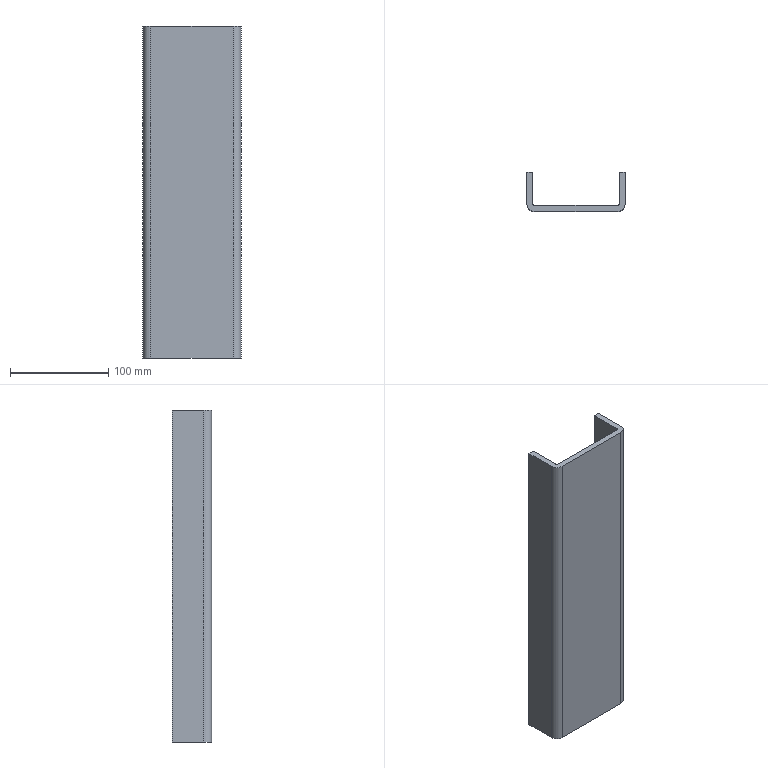Part | SolidWorks | features Extrusion 1 | 1 solid | 14 faces | box 100 x 40 x 337.5 mm | volume 331509 mm3 | plane 10 | cylinder 4 | commonest cylinder face diameters 4 x2 16 x2
STEP:
#1=CARTESIAN_POINT('',(100.,-32.,0.));
#2=VERTEX_POINT('',#1);
#3=CARTESIAN_POINT('',(100.,0.,0.));
#4=VERTEX_POINT('',#3);
#5=CARTESIAN_POINT('',(100.,-32.,0.));
#6=DIRECTION('',(0.,1.,0.));
#7=VECTOR('',#6,1000.);
#8=LINE('',#5,#7);
#9=EDGE_CURVE('',#2,#4,#8,.T.);
#10=ORIENTED_EDGE('',*,*,#9,.T.);
#11=CARTESIAN_POINT('',(100.,0.,337.5));
#12=VERTEX_POINT('',#11);
#13=CARTESIAN_POINT('',(100.,0.,337.5));
#14=DIRECTION('',(0.,0.,-1.));
#15=VECTOR('',#14,1000.);
#16=LINE('',#13,#15);
#17=EDGE_CURVE('',#12,#4,#16,.T.);
#18=ORIENTED_EDGE('',*,*,#17,.F.);
#19=CARTESIAN_POINT('',(100.,-32.,337.5));
#20=VERTEX_POINT('',#19);
#21=CARTESIAN_POINT('',(100.,-32.,337.5));
#22=DIRECTION('',(0.,1.,0.));
#23=VECTOR('',#22,1000.);
#24=LINE('',#21,#23);
#25=EDGE_CURVE('',#20,#12,#24,.T.);
#26=ORIENTED_EDGE('',*,*,#25,.F.);
#27=CARTESIAN_POINT('',(100.,-32.,337.5));
#28=DIRECTION('',(0.,0.,-1.));
#29=VECTOR('',#28,1000.);
#30=LINE('',#27,#29);
#31=EDGE_CURVE('',#20,#2,#30,.T.);
#32=ORIENTED_EDGE('',*,*,#31,.T.);
#33=EDGE_LOOP('',(#10,#18,#26,#32));
#34=FACE_OUTER_BOUND('',#33,.T.);
#35=CARTESIAN_POINT('',(100.,-32.,337.5));
#36=DIRECTION('',(-1.,0.,0.));
#37=DIRECTION('',(0.,0.,1.));
#38=AXIS2_PLACEMENT_3D('',#35,#36,#37);
#39=PLANE('',#38);
#40=ADVANCED_FACE('',(#34),#39,.F.);
#41=CARTESIAN_POINT('',(94.,0.,0.));
#42=VERTEX_POINT('',#41);
#43=CARTESIAN_POINT('',(100.,0.,0.));
#44=DIRECTION('',(-1.,0.,0.));
#45=VECTOR('',#44,1000.);
#46=LINE('',#43,#45);
#47=EDGE_CURVE('',#4,#42,#46,.T.);
#48=ORIENTED_EDGE('',*,*,#47,.T.);
#49=CARTESIAN_POINT('',(94.,0.,337.5));
#50=VERTEX_POINT('',#49);
#51=CARTESIAN_POINT('',(94.,0.,337.5));
#52=DIRECTION('',(0.,0.,-1.));
#53=VECTOR('',#52,1000.);
#54=LINE('',#51,#53);
#55=EDGE_CURVE('',#50,#42,#54,.T.);
#56=ORIENTED_EDGE('',*,*,#55,.F.);
#57=CARTESIAN_POINT('',(100.,0.,337.5));
#58=DIRECTION('',(-1.,0.,0.));
#59=VECTOR('',#58,1000.);
#60=LINE('',#57,#59);
#61=EDGE_CURVE('',#12,#50,#60,.T.);
#62=ORIENTED_EDGE('',*,*,#61,.F.);
#63=ORIENTED_EDGE('',*,*,#17,.T.);
#64=EDGE_LOOP('',(#48,#56,#62,#63));
#65=FACE_OUTER_BOUND('',#64,.T.);
#66=CARTESIAN_POINT('',(100.,0.,337.5));
#67=DIRECTION('',(0.,-1.,0.));
#68=DIRECTION('',(0.,0.,-1.));
#69=AXIS2_PLACEMENT_3D('',#66,#67,#68);
#70=PLANE('',#69);
#71=ADVANCED_FACE('',(#65),#70,.F.);
#72=CARTESIAN_POINT('',(94.,-32.,0.));
#73=VERTEX_POINT('',#72);
#74=CARTESIAN_POINT('',(94.,-32.,0.));
#75=DIRECTION('',(0.,1.,0.));
#76=VECTOR('',#75,1000.);
#77=LINE('',#74,#76);
#78=EDGE_CURVE('',#73,#42,#77,.T.);
#79=ORIENTED_EDGE('',*,*,#78,.F.);
#80=CARTESIAN_POINT('',(94.,-32.,337.5));
#81=VERTEX_POINT('',#80);
#82=CARTESIAN_POINT('',(94.,-32.,337.5));
#83=DIRECTION('',(0.,0.,-1.));
#84=VECTOR('',#83,1000.);
#85=LINE('',#82,#84);
#86=EDGE_CURVE('',#81,#73,#85,.T.);
#87=ORIENTED_EDGE('',*,*,#86,.F.);
#88=CARTESIAN_POINT('',(94.,-32.,337.5));
#89=DIRECTION('',(0.,1.,0.));
#90=VECTOR('',#89,1000.);
#91=LINE('',#88,#90);
#92=EDGE_CURVE('',#81,#50,#91,.T.);
#93=ORIENTED_EDGE('',*,*,#92,.T.);
#94=ORIENTED_EDGE('',*,*,#55,.T.);
#95=EDGE_LOOP('',(#79,#87,#93,#94));
#96=FACE_OUTER_BOUND('',#95,.T.);
#97=CARTESIAN_POINT('',(94.,-32.,337.5));
#98=DIRECTION('',(-1.,0.,0.));
#99=DIRECTION('',(0.,-1.,0.));
#100=AXIS2_PLACEMENT_3D('',#97,#98,#99);
#101=PLANE('',#100);
#102=ADVANCED_FACE('',(#96),#101,.T.);
#103=CARTESIAN_POINT('',(92.,-34.,0.));
#104=VERTEX_POINT('',#103);
#105=CARTESIAN_POINT('',(92.,-32.,0.));
#106=DIRECTION('',(0.,0.,1.));
#107=DIRECTION('',(1.,0.,0.));
#108=AXIS2_PLACEMENT_3D('',#105,#106,#107);
#109=CIRCLE('',#108,2.);
#110=EDGE_CURVE('',#104,#73,#109,.T.);
#111=ORIENTED_EDGE('',*,*,#110,.F.);
#112=CARTESIAN_POINT('',(92.,-34.,337.5));
#113=VERTEX_POINT('',#112);
#114=CARTESIAN_POINT('',(92.,-34.,337.5));
#115=DIRECTION('',(0.,0.,-1.));
#116=VECTOR('',#115,1000.);
#117=LINE('',#114,#116);
#118=EDGE_CURVE('',#113,#104,#117,.T.);
#119=ORIENTED_EDGE('',*,*,#118,.F.);
#120=CARTESIAN_POINT('',(92.,-32.,337.5));
#121=DIRECTION('',(0.,0.,1.));
#122=DIRECTION('',(1.,0.,0.));
#123=AXIS2_PLACEMENT_3D('',#120,#121,#122);
#124=CIRCLE('',#123,2.);
#125=EDGE_CURVE('',#113,#81,#124,.T.);
#126=ORIENTED_EDGE('',*,*,#125,.T.);
#127=ORIENTED_EDGE('',*,*,#86,.T.);
#128=EDGE_LOOP('',(#111,#119,#126,#127));
#129=FACE_OUTER_BOUND('',#128,.T.);
#130=CARTESIAN_POINT('',(92.,-32.,337.5));
#131=DIRECTION('',(0.,0.,-1.));
#132=DIRECTION('',(-1.,0.,0.));
#133=AXIS2_PLACEMENT_3D('',#130,#131,#132);
#134=CYLINDRICAL_SURFACE('',#133,2.);
#135=ADVANCED_FACE('',(#129),#134,.F.);
#136=CARTESIAN_POINT('',(8.,-34.,0.));
#137=VERTEX_POINT('',#136);
#138=CARTESIAN_POINT('',(8.,-34.,0.));
#139=DIRECTION('',(1.,0.,0.));
#140=VECTOR('',#139,1000.);
#141=LINE('',#138,#140);
#142=EDGE_CURVE('',#137,#104,#141,.T.);
#143=ORIENTED_EDGE('',*,*,#142,.F.);
#144=CARTESIAN_POINT('',(8.,-34.,337.5));
#145=VERTEX_POINT('',#144);
#146=CARTESIAN_POINT('',(8.,-34.,337.5));
#147=DIRECTION('',(0.,0.,-1.));
#148=VECTOR('',#147,1000.);
#149=LINE('',#146,#148);
#150=EDGE_CURVE('',#145,#137,#149,.T.);
#151=ORIENTED_EDGE('',*,*,#150,.F.);
#152=CARTESIAN_POINT('',(8.,-34.,337.5));
#153=DIRECTION('',(1.,0.,0.));
#154=VECTOR('',#153,1000.);
#155=LINE('',#152,#154);
#156=EDGE_CURVE('',#145,#113,#155,.T.);
#157=ORIENTED_EDGE('',*,*,#156,.T.);
#158=ORIENTED_EDGE('',*,*,#118,.T.);
#159=EDGE_LOOP('',(#143,#151,#157,#158));
#160=FACE_OUTER_BOUND('',#159,.T.);
#161=CARTESIAN_POINT('',(8.,-34.,337.5));
#162=DIRECTION('',(0.,1.,0.));
#163=DIRECTION('',(0.,0.,1.));
#164=AXIS2_PLACEMENT_3D('',#161,#162,#163);
#165=PLANE('',#164);
#166=ADVANCED_FACE('',(#160),#165,.T.);
#167=CARTESIAN_POINT('',(6.,-32.,0.));
#168=VERTEX_POINT('',#167);
#169=CARTESIAN_POINT('',(8.,-32.,0.));
#170=DIRECTION('',(0.,0.,1.));
#171=DIRECTION('',(1.,0.,0.));
#172=AXIS2_PLACEMENT_3D('',#169,#170,#171);
#173=CIRCLE('',#172,2.);
#174=EDGE_CURVE('',#168,#137,#173,.T.);
#175=ORIENTED_EDGE('',*,*,#174,.F.);
#176=CARTESIAN_POINT('',(6.,-32.,337.5));
#177=VERTEX_POINT('',#176);
#178=CARTESIAN_POINT('',(6.,-32.,337.5));
#179=DIRECTION('',(0.,0.,-1.));
#180=VECTOR('',#179,1000.);
#181=LINE('',#178,#180);
#182=EDGE_CURVE('',#177,#168,#181,.T.);
#183=ORIENTED_EDGE('',*,*,#182,.F.);
#184=CARTESIAN_POINT('',(8.,-32.,337.5));
#185=DIRECTION('',(0.,0.,1.));
#186=DIRECTION('',(1.,0.,0.));
#187=AXIS2_PLACEMENT_3D('',#184,#185,#186);
#188=CIRCLE('',#187,2.);
#189=EDGE_CURVE('',#177,#145,#188,.T.);
#190=ORIENTED_EDGE('',*,*,#189,.T.);
#191=ORIENTED_EDGE('',*,*,#150,.T.);
#192=EDGE_LOOP('',(#175,#183,#190,#191));
#193=FACE_OUTER_BOUND('',#192,.T.);
#194=CARTESIAN_POINT('',(8.,-32.,337.5));
#195=DIRECTION('',(0.,0.,-1.));
#196=DIRECTION('',(-1.,0.,0.));
#197=AXIS2_PLACEMENT_3D('',#194,#195,#196);
#198=CYLINDRICAL_SURFACE('',#197,2.);
#199=ADVANCED_FACE('',(#193),#198,.F.);
#200=CARTESIAN_POINT('',(6.,0.,0.));
#201=VERTEX_POINT('',#200);
#202=CARTESIAN_POINT('',(6.,0.,0.));
#203=DIRECTION('',(0.,-1.,0.));
#204=VECTOR('',#203,1000.);
#205=LINE('',#202,#204);
#206=EDGE_CURVE('',#201,#168,#205,.T.);
#207=ORIENTED_EDGE('',*,*,#206,.F.);
#208=CARTESIAN_POINT('',(6.,0.,337.5));
#209=VERTEX_POINT('',#208);
#210=CARTESIAN_POINT('',(6.,0.,337.5));
#211=DIRECTION('',(0.,0.,-1.));
#212=VECTOR('',#211,1000.);
#213=LINE('',#210,#212);
#214=EDGE_CURVE('',#209,#201,#213,.T.);
#215=ORIENTED_EDGE('',*,*,#214,.F.);
#216=CARTESIAN_POINT('',(6.,0.,337.5));
#217=DIRECTION('',(0.,-1.,0.));
#218=VECTOR('',#217,1000.);
#219=LINE('',#216,#218);
#220=EDGE_CURVE('',#209,#177,#219,.T.);
#221=ORIENTED_EDGE('',*,*,#220,.T.);
#222=ORIENTED_EDGE('',*,*,#182,.T.);
#223=EDGE_LOOP('',(#207,#215,#221,#222));
#224=FACE_OUTER_BOUND('',#223,.T.);
#225=CARTESIAN_POINT('',(6.,0.,337.5));
#226=DIRECTION('',(1.,0.,0.));
#227=DIRECTION('',(0.,0.,-1.));
#228=AXIS2_PLACEMENT_3D('',#225,#226,#227);
#229=PLANE('',#228);
#230=ADVANCED_FACE('',(#224),#229,.T.);
#231=CARTESIAN_POINT('',(0.,0.,0.));
#232=VERTEX_POINT('',#231);
#233=CARTESIAN_POINT('',(6.,0.,0.));
#234=DIRECTION('',(-1.,0.,0.));
#235=VECTOR('',#234,1000.);
#236=LINE('',#233,#235);
#237=EDGE_CURVE('',#201,#232,#236,.T.);
#238=ORIENTED_EDGE('',*,*,#237,.T.);
#239=CARTESIAN_POINT('',(0.,0.,337.5));
#240=VERTEX_POINT('',#239);
#241=CARTESIAN_POINT('',(0.,0.,337.5));
#242=DIRECTION('',(0.,0.,-1.));
#243=VECTOR('',#242,1000.);
#244=LINE('',#241,#243);
#245=EDGE_CURVE('',#240,#232,#244,.T.);
#246=ORIENTED_EDGE('',*,*,#245,.F.);
#247=CARTESIAN_POINT('',(6.,0.,337.5));
#248=DIRECTION('',(-1.,0.,0.));
#249=VECTOR('',#248,1000.);
#250=LINE('',#247,#249);
#251=EDGE_CURVE('',#209,#240,#250,.T.);
#252=ORIENTED_EDGE('',*,*,#251,.F.);
#253=ORIENTED_EDGE('',*,*,#214,.T.);
#254=EDGE_LOOP('',(#238,#246,#252,#253));
#255=FACE_OUTER_BOUND('',#254,.T.);
#256=CARTESIAN_POINT('',(6.,0.,337.5));
#257=DIRECTION('',(0.,-1.,0.));
#258=DIRECTION('',(0.,0.,-1.));
#259=AXIS2_PLACEMENT_3D('',#256,#257,#258);
#260=PLANE('',#259);
#261=ADVANCED_FACE('',(#255),#260,.F.);
#262=CARTESIAN_POINT('',(0.,-32.,0.));
#263=VERTEX_POINT('',#262);
#264=CARTESIAN_POINT('',(0.,0.,0.));
#265=DIRECTION('',(0.,-1.,0.));
#266=VECTOR('',#265,1000.);
#267=LINE('',#264,#266);
#268=EDGE_CURVE('',#232,#263,#267,.T.);
#269=ORIENTED_EDGE('',*,*,#268,.T.);
#270=CARTESIAN_POINT('',(0.,-32.,337.5));
#271=VERTEX_POINT('',#270);
#272=CARTESIAN_POINT('',(0.,-32.,337.5));
#273=DIRECTION('',(0.,0.,-1.));
#274=VECTOR('',#273,1000.);
#275=LINE('',#272,#274);
#276=EDGE_CURVE('',#271,#263,#275,.T.);
#277=ORIENTED_EDGE('',*,*,#276,.F.);
#278=CARTESIAN_POINT('',(0.,0.,337.5));
#279=DIRECTION('',(0.,-1.,0.));
#280=VECTOR('',#279,1000.);
#281=LINE('',#278,#280);
#282=EDGE_CURVE('',#240,#271,#281,.T.);
#283=ORIENTED_EDGE('',*,*,#282,.F.);
#284=ORIENTED_EDGE('',*,*,#245,.T.);
#285=EDGE_LOOP('',(#269,#277,#283,#284));
#286=FACE_OUTER_BOUND('',#285,.T.);
#287=CARTESIAN_POINT('',(0.,0.,337.5));
#288=DIRECTION('',(1.,0.,0.));
#289=DIRECTION('',(0.,0.,-1.));
#290=AXIS2_PLACEMENT_3D('',#287,#288,#289);
#291=PLANE('',#290);
#292=ADVANCED_FACE('',(#286),#291,.F.);
#293=CARTESIAN_POINT('',(8.,-40.,0.));
#294=VERTEX_POINT('',#293);
#295=CARTESIAN_POINT('',(8.,-32.,0.));
#296=DIRECTION('',(0.,0.,1.));
#297=DIRECTION('',(1.,0.,0.));
#298=AXIS2_PLACEMENT_3D('',#295,#296,#297);
#299=CIRCLE('',#298,8.);
#300=EDGE_CURVE('',#263,#294,#299,.T.);
#301=ORIENTED_EDGE('',*,*,#300,.T.);
#302=CARTESIAN_POINT('',(8.,-40.,337.5));
#303=VERTEX_POINT('',#302);
#304=CARTESIAN_POINT('',(8.,-40.,337.5));
#305=DIRECTION('',(0.,0.,-1.));
#306=VECTOR('',#305,1000.);
#307=LINE('',#304,#306);
#308=EDGE_CURVE('',#303,#294,#307,.T.);
#309=ORIENTED_EDGE('',*,*,#308,.F.);
#310=CARTESIAN_POINT('',(8.,-32.,337.5));
#311=DIRECTION('',(0.,0.,1.));
#312=DIRECTION('',(1.,0.,0.));
#313=AXIS2_PLACEMENT_3D('',#310,#311,#312);
#314=CIRCLE('',#313,8.);
#315=EDGE_CURVE('',#271,#303,#314,.T.);
#316=ORIENTED_EDGE('',*,*,#315,.F.);
#317=ORIENTED_EDGE('',*,*,#276,.T.);
#318=EDGE_LOOP('',(#301,#309,#316,#317));
#319=FACE_OUTER_BOUND('',#318,.T.);
#320=CARTESIAN_POINT('',(8.,-32.,337.5));
#321=DIRECTION('',(0.,0.,-1.));
#322=DIRECTION('',(-1.,0.,0.));
#323=AXIS2_PLACEMENT_3D('',#320,#321,#322);
#324=CYLINDRICAL_SURFACE('',#323,8.);
#325=ADVANCED_FACE('',(#319),#324,.T.);
#326=CARTESIAN_POINT('',(92.,-40.,0.));
#327=VERTEX_POINT('',#326);
#328=CARTESIAN_POINT('',(8.,-40.,0.));
#329=DIRECTION('',(1.,0.,0.));
#330=VECTOR('',#329,1000.);
#331=LINE('',#328,#330);
#332=EDGE_CURVE('',#294,#327,#331,.T.);
#333=ORIENTED_EDGE('',*,*,#332,.T.);
#334=CARTESIAN_POINT('',(92.,-40.,337.5));
#335=VERTEX_POINT('',#334);
#336=CARTESIAN_POINT('',(92.,-40.,337.5));
#337=DIRECTION('',(0.,0.,-1.));
#338=VECTOR('',#337,1000.);
#339=LINE('',#336,#338);
#340=EDGE_CURVE('',#335,#327,#339,.T.);
#341=ORIENTED_EDGE('',*,*,#340,.F.);
#342=CARTESIAN_POINT('',(8.,-40.,337.5));
#343=DIRECTION('',(1.,0.,0.));
#344=VECTOR('',#343,1000.);
#345=LINE('',#342,#344);
#346=EDGE_CURVE('',#303,#335,#345,.T.);
#347=ORIENTED_EDGE('',*,*,#346,.F.);
#348=ORIENTED_EDGE('',*,*,#308,.T.);
#349=EDGE_LOOP('',(#333,#341,#347,#348));
#350=FACE_OUTER_BOUND('',#349,.T.);
#351=CARTESIAN_POINT('',(8.,-40.,337.5));
#352=DIRECTION('',(0.,1.,0.));
#353=DIRECTION('',(0.,0.,1.));
#354=AXIS2_PLACEMENT_3D('',#351,#352,#353);
#355=PLANE('',#354);
#356=ADVANCED_FACE('',(#350),#355,.F.);
#357=CARTESIAN_POINT('',(92.,-32.,0.));
#358=DIRECTION('',(0.,0.,1.));
#359=DIRECTION('',(1.,0.,0.));
#360=AXIS2_PLACEMENT_3D('',#357,#358,#359);
#361=CIRCLE('',#360,8.);
#362=EDGE_CURVE('',#327,#2,#361,.T.);
#363=ORIENTED_EDGE('',*,*,#362,.T.);
#364=ORIENTED_EDGE('',*,*,#31,.F.);
#365=CARTESIAN_POINT('',(92.,-32.,337.5));
#366=DIRECTION('',(0.,0.,1.));
#367=DIRECTION('',(1.,0.,0.));
#368=AXIS2_PLACEMENT_3D('',#365,#366,#367);
#369=CIRCLE('',#368,8.);
#370=EDGE_CURVE('',#335,#20,#369,.T.);
#371=ORIENTED_EDGE('',*,*,#370,.F.);
#372=ORIENTED_EDGE('',*,*,#340,.T.);
#373=EDGE_LOOP('',(#363,#364,#371,#372));
#374=FACE_OUTER_BOUND('',#373,.T.);
#375=CARTESIAN_POINT('',(92.,-32.,337.5));
#376=DIRECTION('',(0.,0.,-1.));
#377=DIRECTION('',(-1.,0.,0.));
#378=AXIS2_PLACEMENT_3D('',#375,#376,#377);
#379=CYLINDRICAL_SURFACE('',#378,8.);
#380=ADVANCED_FACE('',(#374),#379,.T.);
#381=ORIENTED_EDGE('',*,*,#25,.T.);
#382=ORIENTED_EDGE('',*,*,#61,.T.);
#383=ORIENTED_EDGE('',*,*,#92,.F.);
#384=ORIENTED_EDGE('',*,*,#125,.F.);
#385=ORIENTED_EDGE('',*,*,#156,.F.);
#386=ORIENTED_EDGE('',*,*,#189,.F.);
#387=ORIENTED_EDGE('',*,*,#220,.F.);
#388=ORIENTED_EDGE('',*,*,#251,.T.);
#389=ORIENTED_EDGE('',*,*,#282,.T.);
#390=ORIENTED_EDGE('',*,*,#315,.T.);
#391=ORIENTED_EDGE('',*,*,#346,.T.);
#392=ORIENTED_EDGE('',*,*,#370,.T.);
#393=EDGE_LOOP('',(#381,#382,#383,#384,#385,#386,#387,#388,#389,#390,#391,#392));
#394=FACE_OUTER_BOUND('',#393,.T.);
#395=CARTESIAN_POINT('',(92.,-32.,337.5));
#396=DIRECTION('',(0.,0.,1.));
#397=DIRECTION('',(1.,0.,0.));
#398=AXIS2_PLACEMENT_3D('',#395,#396,#397);
#399=PLANE('',#398);
#400=ADVANCED_FACE('',(#394),#399,.T.);
#401=ORIENTED_EDGE('',*,*,#9,.F.);
#402=ORIENTED_EDGE('',*,*,#362,.F.);
#403=ORIENTED_EDGE('',*,*,#332,.F.);
#404=ORIENTED_EDGE('',*,*,#300,.F.);
#405=ORIENTED_EDGE('',*,*,#268,.F.);
#406=ORIENTED_EDGE('',*,*,#237,.F.);
#407=ORIENTED_EDGE('',*,*,#206,.T.);
#408=ORIENTED_EDGE('',*,*,#174,.T.);
#409=ORIENTED_EDGE('',*,*,#142,.T.);
#410=ORIENTED_EDGE('',*,*,#110,.T.);
#411=ORIENTED_EDGE('',*,*,#78,.T.);
#412=ORIENTED_EDGE('',*,*,#47,.F.);
#413=EDGE_LOOP('',(#401,#402,#403,#404,#405,#406,#407,#408,#409,#410,#411,#412));
#414=FACE_OUTER_BOUND('',#413,.T.);
#415=CARTESIAN_POINT('',(92.,-32.,0.));
#416=DIRECTION('',(0.,0.,1.));
#417=DIRECTION('',(1.,0.,0.));
#418=AXIS2_PLACEMENT_3D('',#415,#416,#417);
#419=PLANE('',#418);
#420=ADVANCED_FACE('',(#414),#419,.F.);
#421=CLOSED_SHELL('',(#40,#71,#102,#135,#166,#199,#230,#261,#292,#325,#356,#380,#400,#420));
#422=MANIFOLD_SOLID_BREP('',#421);
#423=CARTESIAN_POINT('',(0.,0.,0.));
#424=DIRECTION('',(0.,0.,1.));
#425=DIRECTION('',(1.,0.,0.));
#426=AXIS2_PLACEMENT_3D('',#423,#424,#425);
#427=(LENGTH_UNIT()NAMED_UNIT(*)SI_UNIT(.MILLI.,.METRE.));
#428=UNCERTAINTY_MEASURE_WITH_UNIT(LENGTH_MEASURE(0.00001),#427,'','');
#429=(NAMED_UNIT(*)PLANE_ANGLE_UNIT()SI_UNIT($,.RADIAN.));
#430=(NAMED_UNIT(*)SI_UNIT($,.STERADIAN.)SOLID_ANGLE_UNIT());
#431=(GEOMETRIC_REPRESENTATION_CONTEXT(3)GLOBAL_UNCERTAINTY_ASSIGNED_CONTEXT((#428))GLOBAL_UNIT_ASSIGNED_CONTEXT((#427,#429,#430))REPRESENTATION_CONTEXT('',''));
#432=ADVANCED_BREP_SHAPE_REPRESENTATION('',(#422,#426),#431);